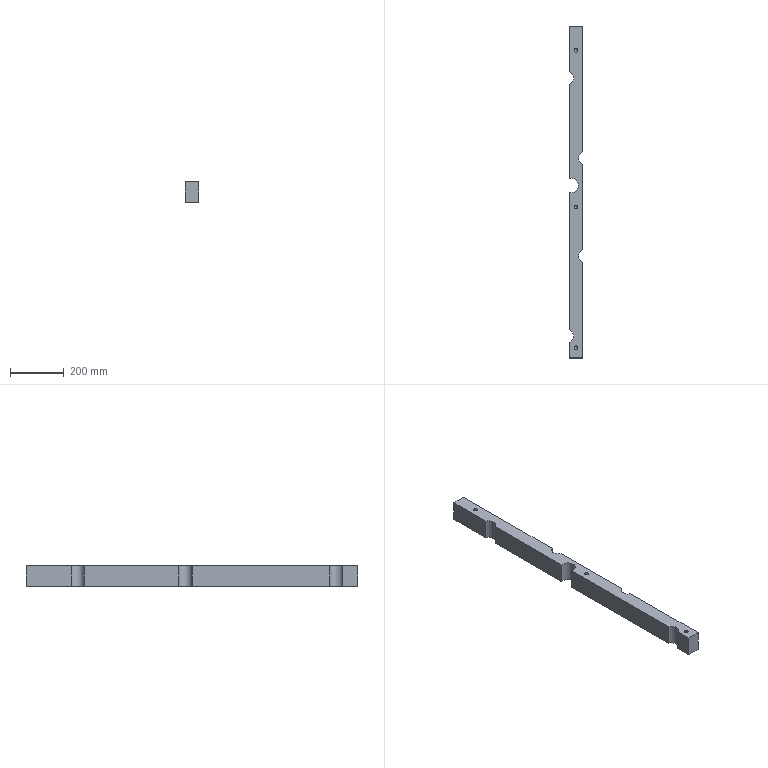Part | NX | features 3 2 | 1 solid | 28 faces | box 50 x 1233 x 75.5 mm | volume 4360512 mm3 | plane 11 | cylinder 11 | cone 6 | commonest cylinder face diameters 14.1 x6 53 x5
STEP:
#1=CARTESIAN_POINT('',(2367.05,582.5,256.5));
#2=VERTEX_POINT('',#1);
#3=CARTESIAN_POINT('',(2360.,582.5,256.5));
#4=DIRECTION('',(0.,0.,-1.));
#5=DIRECTION('',(1.,0.,0.));
#6=AXIS2_PLACEMENT_3D('',#3,#4,#5);
#7=CIRCLE('',#6,7.05);
#8=EDGE_CURVE('',#2,#2,#7,.T.);
#9=ORIENTED_EDGE('',*,*,#8,.T.);
#10=EDGE_LOOP('',(#9));
#11=FACE_BOUND('',#10,.T.);
#12=CARTESIAN_POINT('',(2385.,-157.891,256.5));
#13=VERTEX_POINT('',#12);
#14=CARTESIAN_POINT('',(2385.,157.891,256.5));
#15=VERTEX_POINT('',#14);
#16=CARTESIAN_POINT('',(2385.,193.,256.5));
#17=DIRECTION('',(0.,1.,0.));
#18=VECTOR('',#17,1000.);
#19=LINE('',#16,#18);
#20=EDGE_CURVE('',#13,#15,#19,.T.);
#21=ORIENTED_EDGE('',*,*,#20,.T.);
#22=CARTESIAN_POINT('',(2385.,206.109,256.5));
#23=VERTEX_POINT('',#22);
#24=CARTESIAN_POINT('',(2396.,182.,256.5));
#25=DIRECTION('',(0.,0.,1.));
#26=DIRECTION('',(1.,0.,0.));
#27=AXIS2_PLACEMENT_3D('',#24,#25,#26);
#28=CIRCLE('',#27,26.5);
#29=EDGE_CURVE('',#23,#15,#28,.T.);
#30=ORIENTED_EDGE('',*,*,#29,.F.);
#31=CARTESIAN_POINT('',(2385.,672.5,256.5));
#32=VERTEX_POINT('',#31);
#33=CARTESIAN_POINT('',(2385.,193.,256.5));
#34=DIRECTION('',(0.,1.,0.));
#35=VECTOR('',#34,1000.);
#36=LINE('',#33,#35);
#37=EDGE_CURVE('',#23,#32,#36,.T.);
#38=ORIENTED_EDGE('',*,*,#37,.T.);
#39=CARTESIAN_POINT('',(2335.,672.5,256.5));
#40=VERTEX_POINT('',#39);
#41=CARTESIAN_POINT('',(345.,672.5,256.5));
#42=DIRECTION('',(-1.,0.,0.));
#43=VECTOR('',#42,1000.);
#44=LINE('',#41,#43);
#45=EDGE_CURVE('',#32,#40,#44,.T.);
#46=ORIENTED_EDGE('',*,*,#45,.T.);
#47=CARTESIAN_POINT('',(2335.,504.541,256.5));
#48=VERTEX_POINT('',#47);
#49=CARTESIAN_POINT('',(2335.,193.,256.5));
#50=DIRECTION('',(0.,-1.,0.));
#51=VECTOR('',#50,1000.);
#52=LINE('',#49,#51);
#53=EDGE_CURVE('',#40,#48,#52,.T.);
#54=ORIENTED_EDGE('',*,*,#53,.T.);
#55=CARTESIAN_POINT('',(2335.,455.459,256.5));
#56=VERTEX_POINT('',#55);
#57=CARTESIAN_POINT('',(2325.,480.,256.5));
#58=DIRECTION('',(0.,0.,-1.));
#59=DIRECTION('',(1.,0.,0.));
#60=AXIS2_PLACEMENT_3D('',#57,#58,#59);
#61=CIRCLE('',#60,26.5);
#62=EDGE_CURVE('',#48,#56,#61,.T.);
#63=ORIENTED_EDGE('',*,*,#62,.T.);
#64=CARTESIAN_POINT('',(2335.,105.264,256.5));
#65=VERTEX_POINT('',#64);
#66=CARTESIAN_POINT('',(2335.,193.,256.5));
#67=DIRECTION('',(0.,-1.,0.));
#68=VECTOR('',#67,1000.);
#69=LINE('',#66,#68);
#70=EDGE_CURVE('',#56,#65,#69,.T.);
#71=ORIENTED_EDGE('',*,*,#70,.T.);
#72=CARTESIAN_POINT('',(2335.,54.736,256.5));
#73=VERTEX_POINT('',#72);
#74=CARTESIAN_POINT('',(2343.,80.,256.5));
#75=DIRECTION('',(0.,0.,-1.));
#76=DIRECTION('',(1.,0.,0.));
#77=AXIS2_PLACEMENT_3D('',#74,#75,#76);
#78=CIRCLE('',#77,26.5);
#79=EDGE_CURVE('',#65,#73,#78,.T.);
#80=ORIENTED_EDGE('',*,*,#79,.T.);
#81=CARTESIAN_POINT('',(2335.,-455.459,256.5));
#82=VERTEX_POINT('',#81);
#83=CARTESIAN_POINT('',(2335.,193.,256.5));
#84=DIRECTION('',(0.,-1.,0.));
#85=VECTOR('',#84,1000.);
#86=LINE('',#83,#85);
#87=EDGE_CURVE('',#73,#82,#86,.T.);
#88=ORIENTED_EDGE('',*,*,#87,.T.);
#89=CARTESIAN_POINT('',(2335.,-504.541,256.5));
#90=VERTEX_POINT('',#89);
#91=CARTESIAN_POINT('',(2325.,-480.,256.5));
#92=DIRECTION('',(0.,0.,1.));
#93=DIRECTION('',(1.,0.,0.));
#94=AXIS2_PLACEMENT_3D('',#91,#92,#93);
#95=CIRCLE('',#94,26.5);
#96=EDGE_CURVE('',#90,#82,#95,.T.);
#97=ORIENTED_EDGE('',*,*,#96,.F.);
#98=CARTESIAN_POINT('',(2335.,-560.5,256.5));
#99=VERTEX_POINT('',#98);
#100=CARTESIAN_POINT('',(2335.,193.,256.5));
#101=DIRECTION('',(0.,-1.,0.));
#102=VECTOR('',#101,1000.);
#103=LINE('',#100,#102);
#104=EDGE_CURVE('',#90,#99,#103,.T.);
#105=ORIENTED_EDGE('',*,*,#104,.T.);
#106=CARTESIAN_POINT('',(2385.,-560.5,256.5));
#107=VERTEX_POINT('',#106);
#108=CARTESIAN_POINT('',(345.,-560.5,256.5));
#109=DIRECTION('',(1.,0.,0.));
#110=VECTOR('',#109,1000.);
#111=LINE('',#108,#110);
#112=EDGE_CURVE('',#99,#107,#111,.T.);
#113=ORIENTED_EDGE('',*,*,#112,.T.);
#114=CARTESIAN_POINT('',(2385.,-206.109,256.5));
#115=VERTEX_POINT('',#114);
#116=CARTESIAN_POINT('',(2385.,193.,256.5));
#117=DIRECTION('',(0.,1.,0.));
#118=VECTOR('',#117,1000.);
#119=LINE('',#116,#118);
#120=EDGE_CURVE('',#107,#115,#119,.T.);
#121=ORIENTED_EDGE('',*,*,#120,.T.);
#122=CARTESIAN_POINT('',(2396.,-182.,256.5));
#123=DIRECTION('',(0.,0.,1.));
#124=DIRECTION('',(1.,0.,0.));
#125=AXIS2_PLACEMENT_3D('',#122,#123,#124);
#126=CIRCLE('',#125,26.5);
#127=EDGE_CURVE('',#13,#115,#126,.T.);
#128=ORIENTED_EDGE('',*,*,#127,.F.);
#129=EDGE_LOOP('',(#21,#30,#38,#46,#54,#63,#71,#80,#88,#97,#105,#113,#121,#128));
#130=FACE_BOUND('',#129,.T.);
#131=CARTESIAN_POINT('',(2367.05,-522.5,256.5));
#132=VERTEX_POINT('',#131);
#133=CARTESIAN_POINT('',(2360.,-522.5,256.5));
#134=DIRECTION('',(0.,0.,-1.));
#135=DIRECTION('',(1.,0.,0.));
#136=AXIS2_PLACEMENT_3D('',#133,#134,#135);
#137=CIRCLE('',#136,7.05);
#138=EDGE_CURVE('',#132,#132,#137,.T.);
#139=ORIENTED_EDGE('',*,*,#138,.T.);
#140=EDGE_LOOP('',(#139));
#141=FACE_BOUND('',#140,.T.);
#142=CARTESIAN_POINT('',(2367.05,0.,256.5));
#143=VERTEX_POINT('',#142);
#144=CARTESIAN_POINT('',(2360.,0.,256.5));
#145=DIRECTION('',(0.,0.,-1.));
#146=DIRECTION('',(1.,0.,0.));
#147=AXIS2_PLACEMENT_3D('',#144,#145,#146);
#148=CIRCLE('',#147,7.05);
#149=EDGE_CURVE('',#143,#143,#148,.T.);
#150=ORIENTED_EDGE('',*,*,#149,.T.);
#151=EDGE_LOOP('',(#150));
#152=FACE_BOUND('',#151,.T.);
#153=CARTESIAN_POINT('',(345.,0.,256.5));
#154=DIRECTION('',(0.,0.,1.));
#155=DIRECTION('',(1.,0.,0.));
#156=AXIS2_PLACEMENT_3D('',#153,#154,#155);
#157=PLANE('',#156);
#158=ADVANCED_FACE('',(#11,#130,#141,#152),#157,.T.);
#159=CARTESIAN_POINT('',(2367.05,0.,181.));
#160=VERTEX_POINT('',#159);
#161=CARTESIAN_POINT('',(2360.,0.,181.));
#162=DIRECTION('',(0.,0.,1.));
#163=DIRECTION('',(1.,0.,0.));
#164=AXIS2_PLACEMENT_3D('',#161,#162,#163);
#165=CIRCLE('',#164,7.05);
#166=EDGE_CURVE('',#160,#160,#165,.T.);
#167=ORIENTED_EDGE('',*,*,#166,.T.);
#168=EDGE_LOOP('',(#167));
#169=FACE_BOUND('',#168,.T.);
#170=CARTESIAN_POINT('',(2385.,672.5,181.));
#171=VERTEX_POINT('',#170);
#172=CARTESIAN_POINT('',(2385.,206.109,181.));
#173=VERTEX_POINT('',#172);
#174=CARTESIAN_POINT('',(2385.,193.,181.));
#175=DIRECTION('',(0.,-1.,0.));
#176=VECTOR('',#175,1000.);
#177=LINE('',#174,#176);
#178=EDGE_CURVE('',#171,#173,#177,.T.);
#179=ORIENTED_EDGE('',*,*,#178,.T.);
#180=CARTESIAN_POINT('',(2385.,157.891,181.));
#181=VERTEX_POINT('',#180);
#182=CARTESIAN_POINT('',(2396.,182.,181.));
#183=DIRECTION('',(0.,0.,-1.));
#184=DIRECTION('',(-1.,0.,0.));
#185=AXIS2_PLACEMENT_3D('',#182,#183,#184);
#186=CIRCLE('',#185,26.5);
#187=EDGE_CURVE('',#181,#173,#186,.T.);
#188=ORIENTED_EDGE('',*,*,#187,.F.);
#189=CARTESIAN_POINT('',(2385.,-157.891,181.));
#190=VERTEX_POINT('',#189);
#191=CARTESIAN_POINT('',(2385.,193.,181.));
#192=DIRECTION('',(0.,-1.,0.));
#193=VECTOR('',#192,1000.);
#194=LINE('',#191,#193);
#195=EDGE_CURVE('',#181,#190,#194,.T.);
#196=ORIENTED_EDGE('',*,*,#195,.T.);
#197=CARTESIAN_POINT('',(2385.,-206.109,181.));
#198=VERTEX_POINT('',#197);
#199=CARTESIAN_POINT('',(2396.,-182.,181.));
#200=DIRECTION('',(0.,0.,-1.));
#201=DIRECTION('',(-1.,0.,0.));
#202=AXIS2_PLACEMENT_3D('',#199,#200,#201);
#203=CIRCLE('',#202,26.5);
#204=EDGE_CURVE('',#198,#190,#203,.T.);
#205=ORIENTED_EDGE('',*,*,#204,.F.);
#206=CARTESIAN_POINT('',(2385.,-560.5,181.));
#207=VERTEX_POINT('',#206);
#208=CARTESIAN_POINT('',(2385.,193.,181.));
#209=DIRECTION('',(0.,-1.,0.));
#210=VECTOR('',#209,1000.);
#211=LINE('',#208,#210);
#212=EDGE_CURVE('',#198,#207,#211,.T.);
#213=ORIENTED_EDGE('',*,*,#212,.T.);
#214=CARTESIAN_POINT('',(2335.,-560.5,181.));
#215=VERTEX_POINT('',#214);
#216=CARTESIAN_POINT('',(1115.,-560.5,181.));
#217=DIRECTION('',(-1.,0.,0.));
#218=VECTOR('',#217,1000.);
#219=LINE('',#216,#218);
#220=EDGE_CURVE('',#207,#215,#219,.T.);
#221=ORIENTED_EDGE('',*,*,#220,.T.);
#222=CARTESIAN_POINT('',(2335.,-504.541,181.));
#223=VERTEX_POINT('',#222);
#224=CARTESIAN_POINT('',(2335.,193.,181.));
#225=DIRECTION('',(0.,1.,0.));
#226=VECTOR('',#225,1000.);
#227=LINE('',#224,#226);
#228=EDGE_CURVE('',#215,#223,#227,.T.);
#229=ORIENTED_EDGE('',*,*,#228,.T.);
#230=CARTESIAN_POINT('',(2335.,-455.459,181.));
#231=VERTEX_POINT('',#230);
#232=CARTESIAN_POINT('',(2325.,-480.,181.));
#233=DIRECTION('',(0.,0.,-1.));
#234=DIRECTION('',(-1.,0.,0.));
#235=AXIS2_PLACEMENT_3D('',#232,#233,#234);
#236=CIRCLE('',#235,26.5);
#237=EDGE_CURVE('',#231,#223,#236,.T.);
#238=ORIENTED_EDGE('',*,*,#237,.F.);
#239=CARTESIAN_POINT('',(2335.,54.736,181.));
#240=VERTEX_POINT('',#239);
#241=CARTESIAN_POINT('',(2335.,193.,181.));
#242=DIRECTION('',(0.,1.,0.));
#243=VECTOR('',#242,1000.);
#244=LINE('',#241,#243);
#245=EDGE_CURVE('',#231,#240,#244,.T.);
#246=ORIENTED_EDGE('',*,*,#245,.T.);
#247=CARTESIAN_POINT('',(2335.,105.264,181.));
#248=VERTEX_POINT('',#247);
#249=CARTESIAN_POINT('',(2343.,80.,181.));
#250=DIRECTION('',(0.,0.,-1.));
#251=DIRECTION('',(-1.,0.,0.));
#252=AXIS2_PLACEMENT_3D('',#249,#250,#251);
#253=CIRCLE('',#252,26.5);
#254=EDGE_CURVE('',#248,#240,#253,.T.);
#255=ORIENTED_EDGE('',*,*,#254,.F.);
#256=CARTESIAN_POINT('',(2335.,455.459,181.));
#257=VERTEX_POINT('',#256);
#258=CARTESIAN_POINT('',(2335.,193.,181.));
#259=DIRECTION('',(0.,1.,0.));
#260=VECTOR('',#259,1000.);
#261=LINE('',#258,#260);
#262=EDGE_CURVE('',#248,#257,#261,.T.);
#263=ORIENTED_EDGE('',*,*,#262,.T.);
#264=CARTESIAN_POINT('',(2335.,504.541,181.));
#265=VERTEX_POINT('',#264);
#266=CARTESIAN_POINT('',(2325.,480.,181.));
#267=DIRECTION('',(0.,0.,1.));
#268=DIRECTION('',(-1.,0.,0.));
#269=AXIS2_PLACEMENT_3D('',#266,#267,#268);
#270=CIRCLE('',#269,26.5);
#271=EDGE_CURVE('',#257,#265,#270,.T.);
#272=ORIENTED_EDGE('',*,*,#271,.T.);
#273=CARTESIAN_POINT('',(2335.,672.5,181.));
#274=VERTEX_POINT('',#273);
#275=CARTESIAN_POINT('',(2335.,193.,181.));
#276=DIRECTION('',(0.,1.,0.));
#277=VECTOR('',#276,1000.);
#278=LINE('',#275,#277);
#279=EDGE_CURVE('',#265,#274,#278,.T.);
#280=ORIENTED_EDGE('',*,*,#279,.T.);
#281=CARTESIAN_POINT('',(2385.,672.5,181.));
#282=DIRECTION('',(-1.,0.,0.));
#283=VECTOR('',#282,1000.);
#284=LINE('',#281,#283);
#285=EDGE_CURVE('',#171,#274,#284,.T.);
#286=ORIENTED_EDGE('',*,*,#285,.F.);
#287=EDGE_LOOP('',(#179,#188,#196,#205,#213,#221,#229,#238,#246,#255,#263,#272,#280,#286));
#288=FACE_BOUND('',#287,.T.);
#289=CARTESIAN_POINT('',(2367.05,-522.5,181.));
#290=VERTEX_POINT('',#289);
#291=CARTESIAN_POINT('',(2360.,-522.5,181.));
#292=DIRECTION('',(0.,0.,1.));
#293=DIRECTION('',(1.,0.,0.));
#294=AXIS2_PLACEMENT_3D('',#291,#292,#293);
#295=CIRCLE('',#294,7.05);
#296=EDGE_CURVE('',#290,#290,#295,.T.);
#297=ORIENTED_EDGE('',*,*,#296,.T.);
#298=EDGE_LOOP('',(#297));
#299=FACE_BOUND('',#298,.T.);
#300=CARTESIAN_POINT('',(2367.05,582.5,181.));
#301=VERTEX_POINT('',#300);
#302=CARTESIAN_POINT('',(2360.,582.5,181.));
#303=DIRECTION('',(0.,0.,1.));
#304=DIRECTION('',(1.,0.,0.));
#305=AXIS2_PLACEMENT_3D('',#302,#303,#304);
#306=CIRCLE('',#305,7.05);
#307=EDGE_CURVE('',#301,#301,#306,.T.);
#308=ORIENTED_EDGE('',*,*,#307,.T.);
#309=EDGE_LOOP('',(#308));
#310=FACE_BOUND('',#309,.T.);
#311=CARTESIAN_POINT('',(1115.,193.,181.));
#312=DIRECTION('',(0.,0.,-1.));
#313=DIRECTION('',(1.,0.,0.));
#314=AXIS2_PLACEMENT_3D('',#311,#312,#313);
#315=PLANE('',#314);
#316=ADVANCED_FACE('',(#169,#288,#299,#310),#315,.T.);
#317=ORIENTED_EDGE('',*,*,#37,.F.);
#318=CARTESIAN_POINT('',(2385.,206.109,-181.));
#319=DIRECTION('',(0.,0.,-1.));
#320=VECTOR('',#319,1000.);
#321=LINE('',#318,#320);
#322=EDGE_CURVE('',#23,#173,#321,.T.);
#323=ORIENTED_EDGE('',*,*,#322,.T.);
#324=ORIENTED_EDGE('',*,*,#178,.F.);
#325=CARTESIAN_POINT('',(2385.,672.5,231.5));
#326=DIRECTION('',(0.,0.,-1.));
#327=VECTOR('',#326,1000.);
#328=LINE('',#325,#327);
#329=EDGE_CURVE('',#32,#171,#328,.T.);
#330=ORIENTED_EDGE('',*,*,#329,.F.);
#331=EDGE_LOOP('',(#317,#323,#324,#330));
#332=FACE_BOUND('',#331,.T.);
#333=CARTESIAN_POINT('',(2385.,193.,-1.5));
#334=DIRECTION('',(1.,0.,0.));
#335=DIRECTION('',(0.,0.,-1.));
#336=AXIS2_PLACEMENT_3D('',#333,#334,#335);
#337=PLANE('',#336);
#338=ADVANCED_FACE('',(#332),#337,.T.);
#339=ORIENTED_EDGE('',*,*,#195,.F.);
#340=CARTESIAN_POINT('',(2385.,157.891,181.));
#341=DIRECTION('',(0.,0.,1.));
#342=VECTOR('',#341,1000.);
#343=LINE('',#340,#342);
#344=EDGE_CURVE('',#181,#15,#343,.T.);
#345=ORIENTED_EDGE('',*,*,#344,.T.);
#346=ORIENTED_EDGE('',*,*,#20,.F.);
#347=CARTESIAN_POINT('',(2385.,-157.891,-181.));
#348=DIRECTION('',(0.,0.,-1.));
#349=VECTOR('',#348,1000.);
#350=LINE('',#347,#349);
#351=EDGE_CURVE('',#13,#190,#350,.T.);
#352=ORIENTED_EDGE('',*,*,#351,.T.);
#353=EDGE_LOOP('',(#339,#345,#346,#352));
#354=FACE_BOUND('',#353,.T.);
#355=CARTESIAN_POINT('',(2385.,193.,-1.5));
#356=DIRECTION('',(1.,0.,0.));
#357=DIRECTION('',(0.,0.,-1.));
#358=AXIS2_PLACEMENT_3D('',#355,#356,#357);
#359=PLANE('',#358);
#360=ADVANCED_FACE('',(#354),#359,.T.);
#361=CARTESIAN_POINT('',(2335.,-504.541,-181.));
#362=DIRECTION('',(0.,0.,-1.));
#363=VECTOR('',#362,1000.);
#364=LINE('',#361,#363);
#365=EDGE_CURVE('',#90,#223,#364,.T.);
#366=ORIENTED_EDGE('',*,*,#365,.T.);
#367=ORIENTED_EDGE('',*,*,#228,.F.);
#368=CARTESIAN_POINT('',(2335.,-560.5,-1.5));
#369=DIRECTION('',(0.,0.,1.));
#370=VECTOR('',#369,1000.);
#371=LINE('',#368,#370);
#372=EDGE_CURVE('',#215,#99,#371,.T.);
#373=ORIENTED_EDGE('',*,*,#372,.T.);
#374=ORIENTED_EDGE('',*,*,#104,.F.);
#375=EDGE_LOOP('',(#366,#367,#373,#374));
#376=FACE_BOUND('',#375,.T.);
#377=CARTESIAN_POINT('',(2335.,193.,-1.5));
#378=DIRECTION('',(-1.,0.,0.));
#379=DIRECTION('',(0.,0.,1.));
#380=AXIS2_PLACEMENT_3D('',#377,#378,#379);
#381=PLANE('',#380);
#382=ADVANCED_FACE('',(#376),#381,.T.);
#383=CARTESIAN_POINT('',(2335.,-455.459,181.));
#384=DIRECTION('',(0.,0.,1.));
#385=VECTOR('',#384,1000.);
#386=LINE('',#383,#385);
#387=EDGE_CURVE('',#231,#82,#386,.T.);
#388=ORIENTED_EDGE('',*,*,#387,.T.);
#389=ORIENTED_EDGE('',*,*,#87,.F.);
#390=CARTESIAN_POINT('',(2335.,54.736,-181.));
#391=DIRECTION('',(0.,0.,1.));
#392=VECTOR('',#391,1000.);
#393=LINE('',#390,#392);
#394=EDGE_CURVE('',#240,#73,#393,.T.);
#395=ORIENTED_EDGE('',*,*,#394,.F.);
#396=ORIENTED_EDGE('',*,*,#245,.F.);
#397=EDGE_LOOP('',(#388,#389,#395,#396));
#398=FACE_BOUND('',#397,.T.);
#399=CARTESIAN_POINT('',(2335.,193.,-1.5));
#400=DIRECTION('',(-1.,0.,0.));
#401=DIRECTION('',(0.,0.,1.));
#402=AXIS2_PLACEMENT_3D('',#399,#400,#401);
#403=PLANE('',#402);
#404=ADVANCED_FACE('',(#398),#403,.T.);
#405=CARTESIAN_POINT('',(2335.,105.264,256.5));
#406=DIRECTION('',(0.,0.,-1.));
#407=VECTOR('',#406,1000.);
#408=LINE('',#405,#407);
#409=EDGE_CURVE('',#65,#248,#408,.T.);
#410=ORIENTED_EDGE('',*,*,#409,.F.);
#411=ORIENTED_EDGE('',*,*,#70,.F.);
#412=CARTESIAN_POINT('',(2335.,455.459,-181.));
#413=DIRECTION('',(0.,0.,1.));
#414=VECTOR('',#413,1000.);
#415=LINE('',#412,#414);
#416=EDGE_CURVE('',#257,#56,#415,.T.);
#417=ORIENTED_EDGE('',*,*,#416,.F.);
#418=ORIENTED_EDGE('',*,*,#262,.F.);
#419=EDGE_LOOP('',(#410,#411,#417,#418));
#420=FACE_BOUND('',#419,.T.);
#421=CARTESIAN_POINT('',(2335.,193.,-1.5));
#422=DIRECTION('',(-1.,0.,0.));
#423=DIRECTION('',(0.,0.,1.));
#424=AXIS2_PLACEMENT_3D('',#421,#422,#423);
#425=PLANE('',#424);
#426=ADVANCED_FACE('',(#420),#425,.T.);
#427=ORIENTED_EDGE('',*,*,#112,.F.);
#428=ORIENTED_EDGE('',*,*,#372,.F.);
#429=ORIENTED_EDGE('',*,*,#220,.F.);
#430=CARTESIAN_POINT('',(2385.,-560.5,-1.5));
#431=DIRECTION('',(0.,0.,-1.));
#432=VECTOR('',#431,1000.);
#433=LINE('',#430,#432);
#434=EDGE_CURVE('',#107,#207,#433,.T.);
#435=ORIENTED_EDGE('',*,*,#434,.F.);
#436=EDGE_LOOP('',(#427,#428,#429,#435));
#437=FACE_BOUND('',#436,.T.);
#438=CARTESIAN_POINT('',(2415.,-560.5,179.));
#439=DIRECTION('',(0.,-1.,0.));
#440=DIRECTION('',(-1.,0.,0.));
#441=AXIS2_PLACEMENT_3D('',#438,#439,#440);
#442=PLANE('',#441);
#443=ADVANCED_FACE('',(#437),#442,.T.);
#444=CARTESIAN_POINT('',(2385.,-206.109,181.));
#445=DIRECTION('',(0.,0.,1.));
#446=VECTOR('',#445,1000.);
#447=LINE('',#444,#446);
#448=EDGE_CURVE('',#198,#115,#447,.T.);
#449=ORIENTED_EDGE('',*,*,#448,.T.);
#450=ORIENTED_EDGE('',*,*,#120,.F.);
#451=ORIENTED_EDGE('',*,*,#434,.T.);
#452=ORIENTED_EDGE('',*,*,#212,.F.);
#453=EDGE_LOOP('',(#449,#450,#451,#452));
#454=FACE_BOUND('',#453,.T.);
#455=CARTESIAN_POINT('',(2385.,193.,-1.5));
#456=DIRECTION('',(1.,0.,0.));
#457=DIRECTION('',(0.,0.,-1.));
#458=AXIS2_PLACEMENT_3D('',#455,#456,#457);
#459=PLANE('',#458);
#460=ADVANCED_FACE('',(#454),#459,.T.);
#461=CARTESIAN_POINT('',(2335.,504.541,256.5));
#462=DIRECTION('',(0.,0.,-1.));
#463=VECTOR('',#462,1000.);
#464=LINE('',#461,#463);
#465=EDGE_CURVE('',#48,#265,#464,.T.);
#466=ORIENTED_EDGE('',*,*,#465,.F.);
#467=ORIENTED_EDGE('',*,*,#53,.F.);
#468=CARTESIAN_POINT('',(2335.,672.5,231.5));
#469=DIRECTION('',(0.,0.,1.));
#470=VECTOR('',#469,1000.);
#471=LINE('',#468,#470);
#472=EDGE_CURVE('',#274,#40,#471,.T.);
#473=ORIENTED_EDGE('',*,*,#472,.F.);
#474=ORIENTED_EDGE('',*,*,#279,.F.);
#475=EDGE_LOOP('',(#466,#467,#473,#474));
#476=FACE_BOUND('',#475,.T.);
#477=CARTESIAN_POINT('',(2335.,193.,-1.5));
#478=DIRECTION('',(-1.,0.,0.));
#479=DIRECTION('',(0.,0.,1.));
#480=AXIS2_PLACEMENT_3D('',#477,#478,#479);
#481=PLANE('',#480);
#482=ADVANCED_FACE('',(#476),#481,.T.);
#483=ORIENTED_EDGE('',*,*,#329,.T.);
#484=ORIENTED_EDGE('',*,*,#285,.T.);
#485=ORIENTED_EDGE('',*,*,#472,.T.);
#486=ORIENTED_EDGE('',*,*,#45,.F.);
#487=EDGE_LOOP('',(#483,#484,#485,#486));
#488=FACE_BOUND('',#487,.T.);
#489=CARTESIAN_POINT('',(2385.,672.5,231.5));
#490=DIRECTION('',(0.,1.,0.));
#491=DIRECTION('',(0.,0.,-1.));
#492=AXIS2_PLACEMENT_3D('',#489,#490,#491);
#493=PLANE('',#492);
#494=ADVANCED_FACE('',(#488),#493,.T.);
#495=ORIENTED_EDGE('',*,*,#62,.F.);
#496=ORIENTED_EDGE('',*,*,#465,.T.);
#497=ORIENTED_EDGE('',*,*,#271,.F.);
#498=ORIENTED_EDGE('',*,*,#416,.T.);
#499=EDGE_LOOP('',(#495,#496,#497,#498));
#500=FACE_BOUND('',#499,.T.);
#501=CARTESIAN_POINT('',(2325.,480.,-181.));
#502=DIRECTION('',(0.,0.,1.));
#503=DIRECTION('',(-1.,0.,0.));
#504=AXIS2_PLACEMENT_3D('',#501,#502,#503);
#505=CYLINDRICAL_SURFACE('',#504,26.5);
#506=ADVANCED_FACE('',(#500),#505,.F.);
#507=ORIENTED_EDGE('',*,*,#79,.F.);
#508=ORIENTED_EDGE('',*,*,#409,.T.);
#509=ORIENTED_EDGE('',*,*,#254,.T.);
#510=ORIENTED_EDGE('',*,*,#394,.T.);
#511=EDGE_LOOP('',(#507,#508,#509,#510));
#512=FACE_BOUND('',#511,.T.);
#513=CARTESIAN_POINT('',(2343.,80.,-181.));
#514=DIRECTION('',(0.,0.,1.));
#515=DIRECTION('',(-1.,0.,0.));
#516=AXIS2_PLACEMENT_3D('',#513,#514,#515);
#517=CYLINDRICAL_SURFACE('',#516,26.5);
#518=ADVANCED_FACE('',(#512),#517,.F.);
#519=ORIENTED_EDGE('',*,*,#96,.T.);
#520=ORIENTED_EDGE('',*,*,#387,.F.);
#521=ORIENTED_EDGE('',*,*,#237,.T.);
#522=ORIENTED_EDGE('',*,*,#365,.F.);
#523=EDGE_LOOP('',(#519,#520,#521,#522));
#524=FACE_BOUND('',#523,.T.);
#525=CARTESIAN_POINT('',(2325.,-480.,-181.));
#526=DIRECTION('',(0.,0.,1.));
#527=DIRECTION('',(-1.,0.,0.));
#528=AXIS2_PLACEMENT_3D('',#525,#526,#527);
#529=CYLINDRICAL_SURFACE('',#528,26.5);
#530=ADVANCED_FACE('',(#524),#529,.F.);
#531=ORIENTED_EDGE('',*,*,#127,.T.);
#532=ORIENTED_EDGE('',*,*,#448,.F.);
#533=ORIENTED_EDGE('',*,*,#204,.T.);
#534=ORIENTED_EDGE('',*,*,#351,.F.);
#535=EDGE_LOOP('',(#531,#532,#533,#534));
#536=FACE_BOUND('',#535,.T.);
#537=CARTESIAN_POINT('',(2396.,-182.,-181.));
#538=DIRECTION('',(0.,0.,1.));
#539=DIRECTION('',(-1.,0.,0.));
#540=AXIS2_PLACEMENT_3D('',#537,#538,#539);
#541=CYLINDRICAL_SURFACE('',#540,26.5);
#542=ADVANCED_FACE('',(#536),#541,.F.);
#543=ORIENTED_EDGE('',*,*,#29,.T.);
#544=ORIENTED_EDGE('',*,*,#344,.F.);
#545=ORIENTED_EDGE('',*,*,#187,.T.);
#546=ORIENTED_EDGE('',*,*,#322,.F.);
#547=EDGE_LOOP('',(#543,#544,#545,#546));
#548=FACE_BOUND('',#547,.T.);
#549=CARTESIAN_POINT('',(2396.,182.,-181.));
#550=DIRECTION('',(0.,0.,1.));
#551=DIRECTION('',(-1.,0.,0.));
#552=AXIS2_PLACEMENT_3D('',#549,#550,#551);
#553=CYLINDRICAL_SURFACE('',#552,26.5);
#554=ADVANCED_FACE('',(#548),#553,.F.);
#555=CARTESIAN_POINT('',(2367.05,-522.5,188.95));
#556=VERTEX_POINT('',#555);
#557=CARTESIAN_POINT('',(2360.,-522.5,188.95));
#558=DIRECTION('',(0.,0.,1.));
#559=DIRECTION('',(1.,0.,0.));
#560=AXIS2_PLACEMENT_3D('',#557,#558,#559);
#561=CIRCLE('',#560,7.05);
#562=EDGE_CURVE('',#556,#556,#561,.T.);
#563=ORIENTED_EDGE('',*,*,#562,.T.);
#564=EDGE_LOOP('',(#563));
#565=FACE_BOUND('',#564,.T.);
#566=ORIENTED_EDGE('',*,*,#296,.F.);
#567=EDGE_LOOP('',(#566));
#568=FACE_BOUND('',#567,.T.);
#569=CARTESIAN_POINT('',(2360.,-522.5,181.));
#570=DIRECTION('',(0.,0.,1.));
#571=DIRECTION('',(-1.,0.,0.));
#572=AXIS2_PLACEMENT_3D('',#569,#570,#571);
#573=CYLINDRICAL_SURFACE('',#572,7.05);
#574=ADVANCED_FACE('',(#565,#568),#573,.F.);
#575=CARTESIAN_POINT('',(2360.,-522.5,196.));
#576=VERTEX_POINT('',#575);
#577=VERTEX_LOOP('',#576);
#578=FACE_BOUND('',#577,.T.);
#579=ORIENTED_EDGE('',*,*,#562,.F.);
#580=EDGE_LOOP('',(#579));
#581=FACE_BOUND('',#580,.T.);
#582=CARTESIAN_POINT('',(2360.,-522.5,188.95));
#583=DIRECTION('',(0.,0.,-1.));
#584=DIRECTION('',(1.,0.,0.));
#585=AXIS2_PLACEMENT_3D('',#582,#583,#584);
#586=CONICAL_SURFACE('',#585,7.05,0.7854);
#587=ADVANCED_FACE('',(#578,#581),#586,.F.);
#588=CARTESIAN_POINT('',(2367.05,0.,188.95));
#589=VERTEX_POINT('',#588);
#590=CARTESIAN_POINT('',(2360.,0.,188.95));
#591=DIRECTION('',(0.,0.,1.));
#592=DIRECTION('',(1.,0.,0.));
#593=AXIS2_PLACEMENT_3D('',#590,#591,#592);
#594=CIRCLE('',#593,7.05);
#595=EDGE_CURVE('',#589,#589,#594,.T.);
#596=ORIENTED_EDGE('',*,*,#595,.T.);
#597=EDGE_LOOP('',(#596));
#598=FACE_BOUND('',#597,.T.);
#599=ORIENTED_EDGE('',*,*,#166,.F.);
#600=EDGE_LOOP('',(#599));
#601=FACE_BOUND('',#600,.T.);
#602=CARTESIAN_POINT('',(2360.,0.,181.));
#603=DIRECTION('',(0.,0.,1.));
#604=DIRECTION('',(-1.,0.,0.));
#605=AXIS2_PLACEMENT_3D('',#602,#603,#604);
#606=CYLINDRICAL_SURFACE('',#605,7.05);
#607=ADVANCED_FACE('',(#598,#601),#606,.F.);
#608=CARTESIAN_POINT('',(2360.,0.,196.));
#609=VERTEX_POINT('',#608);
#610=VERTEX_LOOP('',#609);
#611=FACE_BOUND('',#610,.T.);
#612=ORIENTED_EDGE('',*,*,#595,.F.);
#613=EDGE_LOOP('',(#612));
#614=FACE_BOUND('',#613,.T.);
#615=CARTESIAN_POINT('',(2360.,0.,188.95));
#616=DIRECTION('',(0.,0.,-1.));
#617=DIRECTION('',(1.,0.,0.));
#618=AXIS2_PLACEMENT_3D('',#615,#616,#617);
#619=CONICAL_SURFACE('',#618,7.05,0.7854);
#620=ADVANCED_FACE('',(#611,#614),#619,.F.);
#621=CARTESIAN_POINT('',(2367.05,582.5,188.95));
#622=VERTEX_POINT('',#621);
#623=CARTESIAN_POINT('',(2360.,582.5,188.95));
#624=DIRECTION('',(0.,0.,1.));
#625=DIRECTION('',(1.,0.,0.));
#626=AXIS2_PLACEMENT_3D('',#623,#624,#625);
#627=CIRCLE('',#626,7.05);
#628=EDGE_CURVE('',#622,#622,#627,.T.);
#629=ORIENTED_EDGE('',*,*,#628,.T.);
#630=EDGE_LOOP('',(#629));
#631=FACE_BOUND('',#630,.T.);
#632=ORIENTED_EDGE('',*,*,#307,.F.);
#633=EDGE_LOOP('',(#632));
#634=FACE_BOUND('',#633,.T.);
#635=CARTESIAN_POINT('',(2360.,582.5,181.));
#636=DIRECTION('',(0.,0.,1.));
#637=DIRECTION('',(-1.,0.,0.));
#638=AXIS2_PLACEMENT_3D('',#635,#636,#637);
#639=CYLINDRICAL_SURFACE('',#638,7.05);
#640=ADVANCED_FACE('',(#631,#634),#639,.F.);
#641=CARTESIAN_POINT('',(2360.,582.5,196.));
#642=VERTEX_POINT('',#641);
#643=VERTEX_LOOP('',#642);
#644=FACE_BOUND('',#643,.T.);
#645=ORIENTED_EDGE('',*,*,#628,.F.);
#646=EDGE_LOOP('',(#645));
#647=FACE_BOUND('',#646,.T.);
#648=CARTESIAN_POINT('',(2360.,582.5,188.95));
#649=DIRECTION('',(0.,0.,-1.));
#650=DIRECTION('',(1.,0.,0.));
#651=AXIS2_PLACEMENT_3D('',#648,#649,#650);
#652=CONICAL_SURFACE('',#651,7.05,0.7854);
#653=ADVANCED_FACE('',(#644,#647),#652,.F.);
#654=CARTESIAN_POINT('',(2352.95,-522.5,248.55));
#655=VERTEX_POINT('',#654);
#656=CARTESIAN_POINT('',(2360.,-522.5,248.55));
#657=DIRECTION('',(0.,0.,-1.));
#658=DIRECTION('',(-1.,0.,0.));
#659=AXIS2_PLACEMENT_3D('',#656,#657,#658);
#660=CIRCLE('',#659,7.05);
#661=EDGE_CURVE('',#655,#655,#660,.T.);
#662=ORIENTED_EDGE('',*,*,#661,.T.);
#663=EDGE_LOOP('',(#662));
#664=FACE_BOUND('',#663,.T.);
#665=ORIENTED_EDGE('',*,*,#138,.F.);
#666=EDGE_LOOP('',(#665));
#667=FACE_BOUND('',#666,.T.);
#668=CARTESIAN_POINT('',(2360.,-522.5,256.5));
#669=DIRECTION('',(0.,0.,-1.));
#670=DIRECTION('',(-1.,0.,0.));
#671=AXIS2_PLACEMENT_3D('',#668,#669,#670);
#672=CYLINDRICAL_SURFACE('',#671,7.05);
#673=ADVANCED_FACE('',(#664,#667),#672,.F.);
#674=CARTESIAN_POINT('',(2360.,-522.5,241.5));
#675=VERTEX_POINT('',#674);
#676=VERTEX_LOOP('',#675);
#677=FACE_BOUND('',#676,.T.);
#678=ORIENTED_EDGE('',*,*,#661,.F.);
#679=EDGE_LOOP('',(#678));
#680=FACE_BOUND('',#679,.T.);
#681=CARTESIAN_POINT('',(2360.,-522.5,248.55));
#682=DIRECTION('',(0.,0.,1.));
#683=DIRECTION('',(-1.,0.,0.));
#684=AXIS2_PLACEMENT_3D('',#681,#682,#683);
#685=CONICAL_SURFACE('',#684,7.05,0.7854);
#686=ADVANCED_FACE('',(#677,#680),#685,.F.);
#687=CARTESIAN_POINT('',(2352.95,582.5,248.55));
#688=VERTEX_POINT('',#687);
#689=CARTESIAN_POINT('',(2360.,582.5,248.55));
#690=DIRECTION('',(0.,0.,-1.));
#691=DIRECTION('',(-1.,0.,0.));
#692=AXIS2_PLACEMENT_3D('',#689,#690,#691);
#693=CIRCLE('',#692,7.05);
#694=EDGE_CURVE('',#688,#688,#693,.T.);
#695=ORIENTED_EDGE('',*,*,#694,.T.);
#696=EDGE_LOOP('',(#695));
#697=FACE_BOUND('',#696,.T.);
#698=ORIENTED_EDGE('',*,*,#8,.F.);
#699=EDGE_LOOP('',(#698));
#700=FACE_BOUND('',#699,.T.);
#701=CARTESIAN_POINT('',(2360.,582.5,256.5));
#702=DIRECTION('',(0.,0.,-1.));
#703=DIRECTION('',(-1.,0.,0.));
#704=AXIS2_PLACEMENT_3D('',#701,#702,#703);
#705=CYLINDRICAL_SURFACE('',#704,7.05);
#706=ADVANCED_FACE('',(#697,#700),#705,.F.);
#707=CARTESIAN_POINT('',(2360.,582.5,241.5));
#708=VERTEX_POINT('',#707);
#709=VERTEX_LOOP('',#708);
#710=FACE_BOUND('',#709,.T.);
#711=ORIENTED_EDGE('',*,*,#694,.F.);
#712=EDGE_LOOP('',(#711));
#713=FACE_BOUND('',#712,.T.);
#714=CARTESIAN_POINT('',(2360.,582.5,248.55));
#715=DIRECTION('',(0.,0.,1.));
#716=DIRECTION('',(-1.,0.,0.));
#717=AXIS2_PLACEMENT_3D('',#714,#715,#716);
#718=CONICAL_SURFACE('',#717,7.05,0.7854);
#719=ADVANCED_FACE('',(#710,#713),#718,.F.);
#720=CARTESIAN_POINT('',(2352.95,0.,248.55));
#721=VERTEX_POINT('',#720);
#722=CARTESIAN_POINT('',(2360.,0.,248.55));
#723=DIRECTION('',(0.,0.,-1.));
#724=DIRECTION('',(-1.,0.,0.));
#725=AXIS2_PLACEMENT_3D('',#722,#723,#724);
#726=CIRCLE('',#725,7.05);
#727=EDGE_CURVE('',#721,#721,#726,.T.);
#728=ORIENTED_EDGE('',*,*,#727,.T.);
#729=EDGE_LOOP('',(#728));
#730=FACE_BOUND('',#729,.T.);
#731=ORIENTED_EDGE('',*,*,#149,.F.);
#732=EDGE_LOOP('',(#731));
#733=FACE_BOUND('',#732,.T.);
#734=CARTESIAN_POINT('',(2360.,0.,256.5));
#735=DIRECTION('',(0.,0.,-1.));
#736=DIRECTION('',(-1.,0.,0.));
#737=AXIS2_PLACEMENT_3D('',#734,#735,#736);
#738=CYLINDRICAL_SURFACE('',#737,7.05);
#739=ADVANCED_FACE('',(#730,#733),#738,.F.);
#740=CARTESIAN_POINT('',(2360.,0.,241.5));
#741=VERTEX_POINT('',#740);
#742=VERTEX_LOOP('',#741);
#743=FACE_BOUND('',#742,.T.);
#744=ORIENTED_EDGE('',*,*,#727,.F.);
#745=EDGE_LOOP('',(#744));
#746=FACE_BOUND('',#745,.T.);
#747=CARTESIAN_POINT('',(2360.,0.,248.55));
#748=DIRECTION('',(0.,0.,1.));
#749=DIRECTION('',(-1.,0.,0.));
#750=AXIS2_PLACEMENT_3D('',#747,#748,#749);
#751=CONICAL_SURFACE('',#750,7.05,0.7854);
#752=ADVANCED_FACE('',(#743,#746),#751,.F.);
#753=CLOSED_SHELL('',(#158,#316,#338,#360,#382,#404,#426,#443,#460,#482,#494,#506,#518,#530,#542,#554,#574,#587,#607,#620,#640,#653,#673,#686,#706,#719,#739,#752));
#754=MANIFOLD_SOLID_BREP('',#753);
#755=(LENGTH_UNIT()NAMED_UNIT(*)SI_UNIT(.MILLI.,.METRE.));
#756=UNCERTAINTY_MEASURE_WITH_UNIT(LENGTH_MEASURE(0.00001),#755,'','');
#757=(NAMED_UNIT(*)PLANE_ANGLE_UNIT()SI_UNIT($,.RADIAN.));
#758=(NAMED_UNIT(*)SI_UNIT($,.STERADIAN.)SOLID_ANGLE_UNIT());
#759=(GEOMETRIC_REPRESENTATION_CONTEXT(3)GLOBAL_UNCERTAINTY_ASSIGNED_CONTEXT((#756))GLOBAL_UNIT_ASSIGNED_CONTEXT((#755,#757,#758))REPRESENTATION_CONTEXT('',''));
#760=ADVANCED_BREP_SHAPE_REPRESENTATION('',(#754),#759);